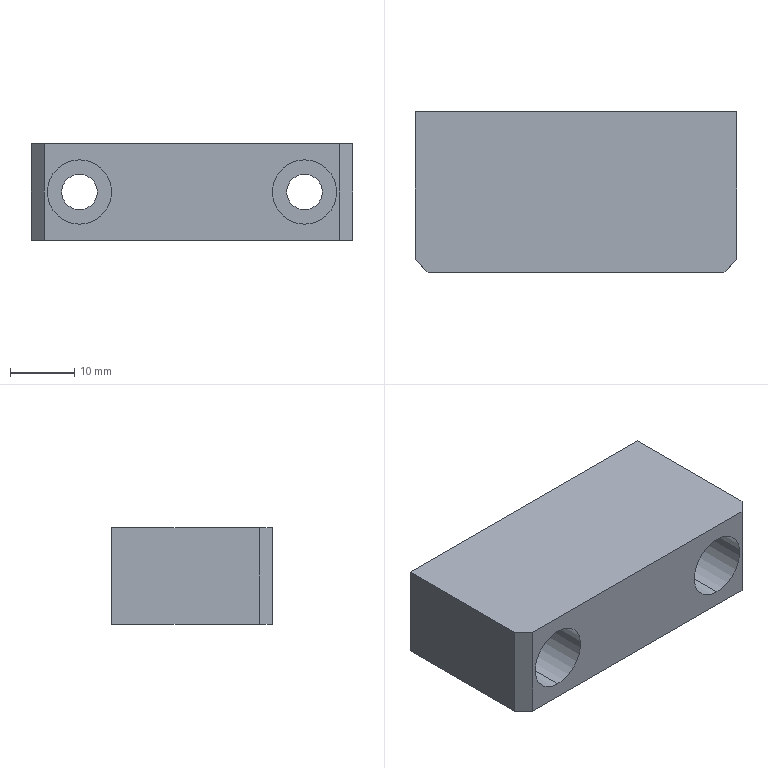Part | SolidWorks | features Chamfer 1, Extrusion 1, HoleWzd 1 | 1 solid | 18 faces | box 50 x 25 x 15 mm | volume 15782 mm3 | plane 10 | cylinder 8 | commonest cylinder face diameters 5.5 x4 10 x4
STEP:
#1=CARTESIAN_POINT('',(17.5,3.2,12.5));
#2=VERTEX_POINT('',#1);
#3=CARTESIAN_POINT('',(17.5,3.2,2.5));
#4=VERTEX_POINT('',#3);
#5=CARTESIAN_POINT('',(17.5,3.2,7.5));
#6=DIRECTION('',(0.,-1.,0.));
#7=DIRECTION('',(0.,0.,-1.));
#8=AXIS2_PLACEMENT_3D('',#5,#6,#7);
#9=CIRCLE('',#8,5.);
#10=EDGE_CURVE('',#2,#4,#9,.T.);
#11=ORIENTED_EDGE('',*,*,#10,.F.);
#12=CARTESIAN_POINT('',(17.5,-12.5,12.5));
#13=VERTEX_POINT('',#12);
#14=CARTESIAN_POINT('',(17.5,-12.5,12.5));
#15=DIRECTION('',(0.,-1.,0.));
#16=VECTOR('',#15,1000.);
#17=LINE('',#14,#16);
#18=EDGE_CURVE('',#2,#13,#17,.T.);
#19=ORIENTED_EDGE('',*,*,#18,.T.);
#20=CARTESIAN_POINT('',(17.5,-12.5,2.5));
#21=VERTEX_POINT('',#20);
#22=CARTESIAN_POINT('',(17.5,-12.5,7.5));
#23=DIRECTION('',(0.,-1.,0.));
#24=DIRECTION('',(0.,0.,-1.));
#25=AXIS2_PLACEMENT_3D('',#22,#23,#24);
#26=CIRCLE('',#25,5.);
#27=EDGE_CURVE('',#13,#21,#26,.T.);
#28=ORIENTED_EDGE('',*,*,#27,.T.);
#29=CARTESIAN_POINT('',(17.5,-12.5,2.5));
#30=DIRECTION('',(0.,-1.,0.));
#31=VECTOR('',#30,1000.);
#32=LINE('',#29,#31);
#33=EDGE_CURVE('',#4,#21,#32,.T.);
#34=ORIENTED_EDGE('',*,*,#33,.F.);
#35=EDGE_LOOP('',(#11,#19,#28,#34));
#36=FACE_OUTER_BOUND('',#35,.T.);
#37=CARTESIAN_POINT('',(17.5,-12.5,7.5));
#38=DIRECTION('',(0.,-1.,0.));
#39=DIRECTION('',(0.,0.,-1.));
#40=AXIS2_PLACEMENT_3D('',#37,#38,#39);
#41=CYLINDRICAL_SURFACE('',#40,5.);
#42=ADVANCED_FACE('',(#36),#41,.F.);
#43=CARTESIAN_POINT('',(17.5,12.5,10.25));
#44=VERTEX_POINT('',#43);
#45=CARTESIAN_POINT('',(17.5,12.5,4.75));
#46=VERTEX_POINT('',#45);
#47=CARTESIAN_POINT('',(17.5,12.5,7.5));
#48=DIRECTION('',(0.,-1.,0.));
#49=DIRECTION('',(0.,0.,-1.));
#50=AXIS2_PLACEMENT_3D('',#47,#48,#49);
#51=CIRCLE('',#50,2.75);
#52=EDGE_CURVE('',#44,#46,#51,.T.);
#53=ORIENTED_EDGE('',*,*,#52,.F.);
#54=CARTESIAN_POINT('',(17.5,3.2,10.25));
#55=VERTEX_POINT('',#54);
#56=CARTESIAN_POINT('',(17.5,-12.5,10.25));
#57=DIRECTION('',(0.,-1.,0.));
#58=VECTOR('',#57,1000.);
#59=LINE('',#56,#58);
#60=EDGE_CURVE('',#44,#55,#59,.T.);
#61=ORIENTED_EDGE('',*,*,#60,.T.);
#62=CARTESIAN_POINT('',(17.5,3.2,4.75));
#63=VERTEX_POINT('',#62);
#64=CARTESIAN_POINT('',(17.5,3.2,7.5));
#65=DIRECTION('',(0.,-1.,0.));
#66=DIRECTION('',(0.,0.,-1.));
#67=AXIS2_PLACEMENT_3D('',#64,#65,#66);
#68=CIRCLE('',#67,2.75);
#69=EDGE_CURVE('',#55,#63,#68,.T.);
#70=ORIENTED_EDGE('',*,*,#69,.T.);
#71=CARTESIAN_POINT('',(17.5,-12.5,4.75));
#72=DIRECTION('',(0.,-1.,0.));
#73=VECTOR('',#72,1000.);
#74=LINE('',#71,#73);
#75=EDGE_CURVE('',#46,#63,#74,.T.);
#76=ORIENTED_EDGE('',*,*,#75,.F.);
#77=EDGE_LOOP('',(#53,#61,#70,#76));
#78=FACE_OUTER_BOUND('',#77,.T.);
#79=CARTESIAN_POINT('',(17.5,-12.5,7.5));
#80=DIRECTION('',(0.,-1.,0.));
#81=DIRECTION('',(0.,0.,-1.));
#82=AXIS2_PLACEMENT_3D('',#79,#80,#81);
#83=CYLINDRICAL_SURFACE('',#82,2.75);
#84=ADVANCED_FACE('',(#78),#83,.F.);
#85=CARTESIAN_POINT('',(-17.5,3.2,12.5));
#86=VERTEX_POINT('',#85);
#87=CARTESIAN_POINT('',(-17.5,3.2,2.5));
#88=VERTEX_POINT('',#87);
#89=CARTESIAN_POINT('',(-17.5,3.2,7.5));
#90=DIRECTION('',(0.,-1.,0.));
#91=DIRECTION('',(0.,0.,-1.));
#92=AXIS2_PLACEMENT_3D('',#89,#90,#91);
#93=CIRCLE('',#92,5.);
#94=EDGE_CURVE('',#86,#88,#93,.T.);
#95=ORIENTED_EDGE('',*,*,#94,.F.);
#96=CARTESIAN_POINT('',(-17.5,-12.5,12.5));
#97=VERTEX_POINT('',#96);
#98=CARTESIAN_POINT('',(-17.5,-12.5,12.5));
#99=DIRECTION('',(0.,-1.,0.));
#100=VECTOR('',#99,1000.);
#101=LINE('',#98,#100);
#102=EDGE_CURVE('',#86,#97,#101,.T.);
#103=ORIENTED_EDGE('',*,*,#102,.T.);
#104=CARTESIAN_POINT('',(-17.5,-12.5,2.5));
#105=VERTEX_POINT('',#104);
#106=CARTESIAN_POINT('',(-17.5,-12.5,7.5));
#107=DIRECTION('',(0.,-1.,0.));
#108=DIRECTION('',(0.,0.,-1.));
#109=AXIS2_PLACEMENT_3D('',#106,#107,#108);
#110=CIRCLE('',#109,5.);
#111=EDGE_CURVE('',#97,#105,#110,.T.);
#112=ORIENTED_EDGE('',*,*,#111,.T.);
#113=CARTESIAN_POINT('',(-17.5,-12.5,2.5));
#114=DIRECTION('',(0.,-1.,0.));
#115=VECTOR('',#114,1000.);
#116=LINE('',#113,#115);
#117=EDGE_CURVE('',#88,#105,#116,.T.);
#118=ORIENTED_EDGE('',*,*,#117,.F.);
#119=EDGE_LOOP('',(#95,#103,#112,#118));
#120=FACE_OUTER_BOUND('',#119,.T.);
#121=CARTESIAN_POINT('',(-17.5,-12.5,7.5));
#122=DIRECTION('',(0.,-1.,0.));
#123=DIRECTION('',(0.,0.,-1.));
#124=AXIS2_PLACEMENT_3D('',#121,#122,#123);
#125=CYLINDRICAL_SURFACE('',#124,5.);
#126=ADVANCED_FACE('',(#120),#125,.F.);
#127=CARTESIAN_POINT('',(-17.5,12.5,10.25));
#128=VERTEX_POINT('',#127);
#129=CARTESIAN_POINT('',(-17.5,12.5,4.75));
#130=VERTEX_POINT('',#129);
#131=CARTESIAN_POINT('',(-17.5,12.5,7.5));
#132=DIRECTION('',(0.,-1.,0.));
#133=DIRECTION('',(0.,0.,-1.));
#134=AXIS2_PLACEMENT_3D('',#131,#132,#133);
#135=CIRCLE('',#134,2.75);
#136=EDGE_CURVE('',#128,#130,#135,.T.);
#137=ORIENTED_EDGE('',*,*,#136,.F.);
#138=CARTESIAN_POINT('',(-17.5,3.2,10.25));
#139=VERTEX_POINT('',#138);
#140=CARTESIAN_POINT('',(-17.5,-12.5,10.25));
#141=DIRECTION('',(0.,-1.,0.));
#142=VECTOR('',#141,1000.);
#143=LINE('',#140,#142);
#144=EDGE_CURVE('',#128,#139,#143,.T.);
#145=ORIENTED_EDGE('',*,*,#144,.T.);
#146=CARTESIAN_POINT('',(-17.5,3.2,4.75));
#147=VERTEX_POINT('',#146);
#148=CARTESIAN_POINT('',(-17.5,3.2,7.5));
#149=DIRECTION('',(0.,-1.,0.));
#150=DIRECTION('',(0.,0.,-1.));
#151=AXIS2_PLACEMENT_3D('',#148,#149,#150);
#152=CIRCLE('',#151,2.75);
#153=EDGE_CURVE('',#139,#147,#152,.T.);
#154=ORIENTED_EDGE('',*,*,#153,.T.);
#155=CARTESIAN_POINT('',(-17.5,-12.5,4.75));
#156=DIRECTION('',(0.,-1.,0.));
#157=VECTOR('',#156,1000.);
#158=LINE('',#155,#157);
#159=EDGE_CURVE('',#130,#147,#158,.T.);
#160=ORIENTED_EDGE('',*,*,#159,.F.);
#161=EDGE_LOOP('',(#137,#145,#154,#160));
#162=FACE_OUTER_BOUND('',#161,.T.);
#163=CARTESIAN_POINT('',(-17.5,-12.5,7.5));
#164=DIRECTION('',(0.,-1.,0.));
#165=DIRECTION('',(0.,0.,-1.));
#166=AXIS2_PLACEMENT_3D('',#163,#164,#165);
#167=CYLINDRICAL_SURFACE('',#166,2.75);
#168=ADVANCED_FACE('',(#162),#167,.F.);
#169=CARTESIAN_POINT('',(25.,-10.5,15.));
#170=VERTEX_POINT('',#169);
#171=CARTESIAN_POINT('',(25.,12.5,15.));
#172=VERTEX_POINT('',#171);
#173=CARTESIAN_POINT('',(25.,-12.5,15.));
#174=DIRECTION('',(0.,1.,0.));
#175=VECTOR('',#174,1000.);
#176=LINE('',#173,#175);
#177=EDGE_CURVE('',#170,#172,#176,.T.);
#178=ORIENTED_EDGE('',*,*,#177,.F.);
#179=CARTESIAN_POINT('',(25.,-10.5,0.));
#180=VERTEX_POINT('',#179);
#181=CARTESIAN_POINT('',(25.,-10.5,15.));
#182=DIRECTION('',(0.,0.,-1.));
#183=VECTOR('',#182,1000.);
#184=LINE('',#181,#183);
#185=EDGE_CURVE('',#170,#180,#184,.T.);
#186=ORIENTED_EDGE('',*,*,#185,.T.);
#187=CARTESIAN_POINT('',(25.,12.5,0.));
#188=VERTEX_POINT('',#187);
#189=CARTESIAN_POINT('',(25.,-12.5,0.));
#190=DIRECTION('',(0.,1.,0.));
#191=VECTOR('',#190,1000.);
#192=LINE('',#189,#191);
#193=EDGE_CURVE('',#180,#188,#192,.T.);
#194=ORIENTED_EDGE('',*,*,#193,.T.);
#195=CARTESIAN_POINT('',(25.,12.5,15.));
#196=DIRECTION('',(0.,0.,-1.));
#197=VECTOR('',#196,1000.);
#198=LINE('',#195,#197);
#199=EDGE_CURVE('',#172,#188,#198,.T.);
#200=ORIENTED_EDGE('',*,*,#199,.F.);
#201=EDGE_LOOP('',(#178,#186,#194,#200));
#202=FACE_OUTER_BOUND('',#201,.T.);
#203=CARTESIAN_POINT('',(25.,-12.5,15.));
#204=DIRECTION('',(-1.,0.,0.));
#205=DIRECTION('',(0.,0.,1.));
#206=AXIS2_PLACEMENT_3D('',#203,#204,#205);
#207=PLANE('',#206);
#208=ADVANCED_FACE('',(#202),#207,.F.);
#209=CARTESIAN_POINT('',(17.5,12.5,7.5));
#210=DIRECTION('',(0.,-1.,0.));
#211=DIRECTION('',(0.,0.,-1.));
#212=AXIS2_PLACEMENT_3D('',#209,#210,#211);
#213=CIRCLE('',#212,2.75);
#214=EDGE_CURVE('',#46,#44,#213,.T.);
#215=ORIENTED_EDGE('',*,*,#214,.T.);
#216=ORIENTED_EDGE('',*,*,#52,.T.);
#217=EDGE_LOOP('',(#215,#216));
#218=FACE_BOUND('',#217,.T.);
#219=CARTESIAN_POINT('',(-17.5,12.5,7.5));
#220=DIRECTION('',(0.,-1.,0.));
#221=DIRECTION('',(0.,0.,-1.));
#222=AXIS2_PLACEMENT_3D('',#219,#220,#221);
#223=CIRCLE('',#222,2.75);
#224=EDGE_CURVE('',#130,#128,#223,.T.);
#225=ORIENTED_EDGE('',*,*,#224,.T.);
#226=ORIENTED_EDGE('',*,*,#136,.T.);
#227=EDGE_LOOP('',(#225,#226));
#228=FACE_BOUND('',#227,.T.);
#229=CARTESIAN_POINT('',(-25.,12.5,0.));
#230=VERTEX_POINT('',#229);
#231=CARTESIAN_POINT('',(-25.,12.5,0.));
#232=DIRECTION('',(-1.,0.,0.));
#233=VECTOR('',#232,1000.);
#234=LINE('',#231,#233);
#235=EDGE_CURVE('',#188,#230,#234,.T.);
#236=ORIENTED_EDGE('',*,*,#235,.T.);
#237=CARTESIAN_POINT('',(-25.,12.5,15.));
#238=VERTEX_POINT('',#237);
#239=CARTESIAN_POINT('',(-25.,12.5,15.));
#240=DIRECTION('',(0.,0.,-1.));
#241=VECTOR('',#240,1000.);
#242=LINE('',#239,#241);
#243=EDGE_CURVE('',#238,#230,#242,.T.);
#244=ORIENTED_EDGE('',*,*,#243,.F.);
#245=CARTESIAN_POINT('',(-25.,12.5,15.));
#246=DIRECTION('',(-1.,0.,0.));
#247=VECTOR('',#246,1000.);
#248=LINE('',#245,#247);
#249=EDGE_CURVE('',#172,#238,#248,.T.);
#250=ORIENTED_EDGE('',*,*,#249,.F.);
#251=ORIENTED_EDGE('',*,*,#199,.T.);
#252=EDGE_LOOP('',(#236,#244,#250,#251));
#253=FACE_OUTER_BOUND('',#252,.T.);
#254=CARTESIAN_POINT('',(-25.,12.5,15.));
#255=DIRECTION('',(0.,-1.,0.));
#256=DIRECTION('',(0.,0.,-1.));
#257=AXIS2_PLACEMENT_3D('',#254,#255,#256);
#258=PLANE('',#257);
#259=ADVANCED_FACE('',(#218,#228,#253),#258,.F.);
#260=CARTESIAN_POINT('',(-25.,-10.5,0.));
#261=VERTEX_POINT('',#260);
#262=CARTESIAN_POINT('',(-25.,-12.5,0.));
#263=DIRECTION('',(0.,-1.,0.));
#264=VECTOR('',#263,1000.);
#265=LINE('',#262,#264);
#266=EDGE_CURVE('',#230,#261,#265,.T.);
#267=ORIENTED_EDGE('',*,*,#266,.T.);
#268=CARTESIAN_POINT('',(-25.,-10.5,15.));
#269=VERTEX_POINT('',#268);
#270=CARTESIAN_POINT('',(-25.,-10.5,15.));
#271=DIRECTION('',(0.,0.,1.));
#272=VECTOR('',#271,1000.);
#273=LINE('',#270,#272);
#274=EDGE_CURVE('',#261,#269,#273,.T.);
#275=ORIENTED_EDGE('',*,*,#274,.T.);
#276=CARTESIAN_POINT('',(-25.,-12.5,15.));
#277=DIRECTION('',(0.,-1.,0.));
#278=VECTOR('',#277,1000.);
#279=LINE('',#276,#278);
#280=EDGE_CURVE('',#238,#269,#279,.T.);
#281=ORIENTED_EDGE('',*,*,#280,.F.);
#282=ORIENTED_EDGE('',*,*,#243,.T.);
#283=EDGE_LOOP('',(#267,#275,#281,#282));
#284=FACE_OUTER_BOUND('',#283,.T.);
#285=CARTESIAN_POINT('',(-25.,-12.5,15.));
#286=DIRECTION('',(1.,0.,0.));
#287=DIRECTION('',(0.,0.,-1.));
#288=AXIS2_PLACEMENT_3D('',#285,#286,#287);
#289=PLANE('',#288);
#290=ADVANCED_FACE('',(#284),#289,.F.);
#291=CARTESIAN_POINT('',(17.5,-12.5,7.5));
#292=DIRECTION('',(0.,-1.,0.));
#293=DIRECTION('',(0.,0.,-1.));
#294=AXIS2_PLACEMENT_3D('',#291,#292,#293);
#295=CIRCLE('',#294,5.);
#296=EDGE_CURVE('',#21,#13,#295,.T.);
#297=ORIENTED_EDGE('',*,*,#296,.F.);
#298=ORIENTED_EDGE('',*,*,#27,.F.);
#299=EDGE_LOOP('',(#297,#298));
#300=FACE_BOUND('',#299,.T.);
#301=CARTESIAN_POINT('',(-17.5,-12.5,7.5));
#302=DIRECTION('',(0.,-1.,0.));
#303=DIRECTION('',(0.,0.,-1.));
#304=AXIS2_PLACEMENT_3D('',#301,#302,#303);
#305=CIRCLE('',#304,5.);
#306=EDGE_CURVE('',#105,#97,#305,.T.);
#307=ORIENTED_EDGE('',*,*,#306,.F.);
#308=ORIENTED_EDGE('',*,*,#111,.F.);
#309=EDGE_LOOP('',(#307,#308));
#310=FACE_BOUND('',#309,.T.);
#311=CARTESIAN_POINT('',(-23.,-12.5,0.));
#312=VERTEX_POINT('',#311);
#313=CARTESIAN_POINT('',(23.,-12.5,0.));
#314=VERTEX_POINT('',#313);
#315=CARTESIAN_POINT('',(-25.,-12.5,0.));
#316=DIRECTION('',(1.,0.,0.));
#317=VECTOR('',#316,1000.);
#318=LINE('',#315,#317);
#319=EDGE_CURVE('',#312,#314,#318,.T.);
#320=ORIENTED_EDGE('',*,*,#319,.T.);
#321=CARTESIAN_POINT('',(23.,-12.5,15.));
#322=VERTEX_POINT('',#321);
#323=CARTESIAN_POINT('',(23.,-12.5,15.));
#324=DIRECTION('',(0.,0.,1.));
#325=VECTOR('',#324,1000.);
#326=LINE('',#323,#325);
#327=EDGE_CURVE('',#314,#322,#326,.T.);
#328=ORIENTED_EDGE('',*,*,#327,.T.);
#329=CARTESIAN_POINT('',(-23.,-12.5,15.));
#330=VERTEX_POINT('',#329);
#331=CARTESIAN_POINT('',(-25.,-12.5,15.));
#332=DIRECTION('',(1.,0.,0.));
#333=VECTOR('',#332,1000.);
#334=LINE('',#331,#333);
#335=EDGE_CURVE('',#330,#322,#334,.T.);
#336=ORIENTED_EDGE('',*,*,#335,.F.);
#337=CARTESIAN_POINT('',(-23.,-12.5,15.));
#338=DIRECTION('',(0.,0.,-1.));
#339=VECTOR('',#338,1000.);
#340=LINE('',#337,#339);
#341=EDGE_CURVE('',#330,#312,#340,.T.);
#342=ORIENTED_EDGE('',*,*,#341,.T.);
#343=EDGE_LOOP('',(#320,#328,#336,#342));
#344=FACE_OUTER_BOUND('',#343,.T.);
#345=CARTESIAN_POINT('',(-25.,-12.5,15.));
#346=DIRECTION('',(0.,1.,0.));
#347=DIRECTION('',(0.,0.,1.));
#348=AXIS2_PLACEMENT_3D('',#345,#346,#347);
#349=PLANE('',#348);
#350=ADVANCED_FACE('',(#300,#310,#344),#349,.F.);
#351=ORIENTED_EDGE('',*,*,#335,.T.);
#352=CARTESIAN_POINT('',(25.,-10.5,15.));
#353=DIRECTION('',(0.7071,0.7071,0.));
#354=VECTOR('',#353,1000.);
#355=LINE('',#352,#354);
#356=EDGE_CURVE('',#322,#170,#355,.T.);
#357=ORIENTED_EDGE('',*,*,#356,.T.);
#358=ORIENTED_EDGE('',*,*,#177,.T.);
#359=ORIENTED_EDGE('',*,*,#249,.T.);
#360=ORIENTED_EDGE('',*,*,#280,.T.);
#361=CARTESIAN_POINT('',(-23.,-12.5,15.));
#362=DIRECTION('',(0.7071,-0.7071,0.));
#363=VECTOR('',#362,1000.);
#364=LINE('',#361,#363);
#365=EDGE_CURVE('',#269,#330,#364,.T.);
#366=ORIENTED_EDGE('',*,*,#365,.T.);
#367=EDGE_LOOP('',(#351,#357,#358,#359,#360,#366));
#368=FACE_OUTER_BOUND('',#367,.T.);
#369=CARTESIAN_POINT('',(0.,0.,15.));
#370=DIRECTION('',(0.,0.,-1.));
#371=DIRECTION('',(-1.,0.,0.));
#372=AXIS2_PLACEMENT_3D('',#369,#370,#371);
#373=PLANE('',#372);
#374=ADVANCED_FACE('',(#368),#373,.F.);
#375=ORIENTED_EDGE('',*,*,#193,.F.);
#376=CARTESIAN_POINT('',(17.75,-17.75,0.));
#377=DIRECTION('',(-0.7071,-0.7071,0.));
#378=VECTOR('',#377,1000.);
#379=LINE('',#376,#378);
#380=EDGE_CURVE('',#180,#314,#379,.T.);
#381=ORIENTED_EDGE('',*,*,#380,.T.);
#382=ORIENTED_EDGE('',*,*,#319,.F.);
#383=CARTESIAN_POINT('',(-17.75,-17.75,0.));
#384=DIRECTION('',(-0.7071,0.7071,0.));
#385=VECTOR('',#384,1000.);
#386=LINE('',#383,#385);
#387=EDGE_CURVE('',#312,#261,#386,.T.);
#388=ORIENTED_EDGE('',*,*,#387,.T.);
#389=ORIENTED_EDGE('',*,*,#266,.F.);
#390=ORIENTED_EDGE('',*,*,#235,.F.);
#391=EDGE_LOOP('',(#375,#381,#382,#388,#389,#390));
#392=FACE_OUTER_BOUND('',#391,.T.);
#393=CARTESIAN_POINT('',(0.,0.,0.));
#394=DIRECTION('',(0.,0.,-1.));
#395=DIRECTION('',(-1.,0.,0.));
#396=AXIS2_PLACEMENT_3D('',#393,#394,#395);
#397=PLANE('',#396);
#398=ADVANCED_FACE('',(#392),#397,.T.);
#399=ORIENTED_EDGE('',*,*,#356,.F.);
#400=ORIENTED_EDGE('',*,*,#327,.F.);
#401=ORIENTED_EDGE('',*,*,#380,.F.);
#402=ORIENTED_EDGE('',*,*,#185,.F.);
#403=EDGE_LOOP('',(#399,#400,#401,#402));
#404=FACE_OUTER_BOUND('',#403,.T.);
#405=CARTESIAN_POINT('',(25.,-10.5,15.));
#406=DIRECTION('',(-0.7071,0.7071,0.));
#407=DIRECTION('',(0.,0.,-1.));
#408=AXIS2_PLACEMENT_3D('',#405,#406,#407);
#409=PLANE('',#408);
#410=ADVANCED_FACE('',(#404),#409,.F.);
#411=ORIENTED_EDGE('',*,*,#365,.F.);
#412=ORIENTED_EDGE('',*,*,#274,.F.);
#413=ORIENTED_EDGE('',*,*,#387,.F.);
#414=ORIENTED_EDGE('',*,*,#341,.F.);
#415=EDGE_LOOP('',(#411,#412,#413,#414));
#416=FACE_OUTER_BOUND('',#415,.T.);
#417=CARTESIAN_POINT('',(-23.,-12.5,15.));
#418=DIRECTION('',(0.7071,0.7071,0.));
#419=DIRECTION('',(0.,0.,-1.));
#420=AXIS2_PLACEMENT_3D('',#417,#418,#419);
#421=PLANE('',#420);
#422=ADVANCED_FACE('',(#416),#421,.F.);
#423=ORIENTED_EDGE('',*,*,#144,.F.);
#424=ORIENTED_EDGE('',*,*,#224,.F.);
#425=ORIENTED_EDGE('',*,*,#159,.T.);
#426=CARTESIAN_POINT('',(-17.5,3.2,7.5));
#427=DIRECTION('',(0.,-1.,0.));
#428=DIRECTION('',(0.,0.,-1.));
#429=AXIS2_PLACEMENT_3D('',#426,#427,#428);
#430=CIRCLE('',#429,2.75);
#431=EDGE_CURVE('',#147,#139,#430,.T.);
#432=ORIENTED_EDGE('',*,*,#431,.T.);
#433=EDGE_LOOP('',(#423,#424,#425,#432));
#434=FACE_OUTER_BOUND('',#433,.T.);
#435=CARTESIAN_POINT('',(-17.5,-12.5,7.5));
#436=DIRECTION('',(0.,-1.,0.));
#437=DIRECTION('',(0.,0.,-1.));
#438=AXIS2_PLACEMENT_3D('',#435,#436,#437);
#439=CYLINDRICAL_SURFACE('',#438,2.75);
#440=ADVANCED_FACE('',(#434),#439,.F.);
#441=ORIENTED_EDGE('',*,*,#431,.F.);
#442=ORIENTED_EDGE('',*,*,#153,.F.);
#443=EDGE_LOOP('',(#441,#442));
#444=FACE_BOUND('',#443,.T.);
#445=CARTESIAN_POINT('',(-17.5,3.2,7.5));
#446=DIRECTION('',(0.,-1.,0.));
#447=DIRECTION('',(0.,0.,-1.));
#448=AXIS2_PLACEMENT_3D('',#445,#446,#447);
#449=CIRCLE('',#448,5.);
#450=EDGE_CURVE('',#88,#86,#449,.T.);
#451=ORIENTED_EDGE('',*,*,#450,.T.);
#452=ORIENTED_EDGE('',*,*,#94,.T.);
#453=EDGE_LOOP('',(#451,#452));
#454=FACE_OUTER_BOUND('',#453,.T.);
#455=CARTESIAN_POINT('',(-14.75,3.2,7.5));
#456=DIRECTION('',(0.,1.,0.));
#457=DIRECTION('',(0.,0.,1.));
#458=AXIS2_PLACEMENT_3D('',#455,#456,#457);
#459=PLANE('',#458);
#460=ADVANCED_FACE('',(#444,#454),#459,.F.);
#461=ORIENTED_EDGE('',*,*,#102,.F.);
#462=ORIENTED_EDGE('',*,*,#450,.F.);
#463=ORIENTED_EDGE('',*,*,#117,.T.);
#464=ORIENTED_EDGE('',*,*,#306,.T.);
#465=EDGE_LOOP('',(#461,#462,#463,#464));
#466=FACE_OUTER_BOUND('',#465,.T.);
#467=CARTESIAN_POINT('',(-17.5,-12.5,7.5));
#468=DIRECTION('',(0.,-1.,0.));
#469=DIRECTION('',(0.,0.,-1.));
#470=AXIS2_PLACEMENT_3D('',#467,#468,#469);
#471=CYLINDRICAL_SURFACE('',#470,5.);
#472=ADVANCED_FACE('',(#466),#471,.F.);
#473=ORIENTED_EDGE('',*,*,#60,.F.);
#474=ORIENTED_EDGE('',*,*,#214,.F.);
#475=ORIENTED_EDGE('',*,*,#75,.T.);
#476=CARTESIAN_POINT('',(17.5,3.2,7.5));
#477=DIRECTION('',(0.,-1.,0.));
#478=DIRECTION('',(0.,0.,-1.));
#479=AXIS2_PLACEMENT_3D('',#476,#477,#478);
#480=CIRCLE('',#479,2.75);
#481=EDGE_CURVE('',#63,#55,#480,.T.);
#482=ORIENTED_EDGE('',*,*,#481,.T.);
#483=EDGE_LOOP('',(#473,#474,#475,#482));
#484=FACE_OUTER_BOUND('',#483,.T.);
#485=CARTESIAN_POINT('',(17.5,-12.5,7.5));
#486=DIRECTION('',(0.,-1.,0.));
#487=DIRECTION('',(0.,0.,-1.));
#488=AXIS2_PLACEMENT_3D('',#485,#486,#487);
#489=CYLINDRICAL_SURFACE('',#488,2.75);
#490=ADVANCED_FACE('',(#484),#489,.F.);
#491=ORIENTED_EDGE('',*,*,#481,.F.);
#492=ORIENTED_EDGE('',*,*,#69,.F.);
#493=EDGE_LOOP('',(#491,#492));
#494=FACE_BOUND('',#493,.T.);
#495=CARTESIAN_POINT('',(17.5,3.2,7.5));
#496=DIRECTION('',(0.,-1.,0.));
#497=DIRECTION('',(0.,0.,-1.));
#498=AXIS2_PLACEMENT_3D('',#495,#496,#497);
#499=CIRCLE('',#498,5.);
#500=EDGE_CURVE('',#4,#2,#499,.T.);
#501=ORIENTED_EDGE('',*,*,#500,.T.);
#502=ORIENTED_EDGE('',*,*,#10,.T.);
#503=EDGE_LOOP('',(#501,#502));
#504=FACE_OUTER_BOUND('',#503,.T.);
#505=CARTESIAN_POINT('',(20.25,3.2,7.5));
#506=DIRECTION('',(0.,1.,0.));
#507=DIRECTION('',(0.,0.,1.));
#508=AXIS2_PLACEMENT_3D('',#505,#506,#507);
#509=PLANE('',#508);
#510=ADVANCED_FACE('',(#494,#504),#509,.F.);
#511=ORIENTED_EDGE('',*,*,#18,.F.);
#512=ORIENTED_EDGE('',*,*,#500,.F.);
#513=ORIENTED_EDGE('',*,*,#33,.T.);
#514=ORIENTED_EDGE('',*,*,#296,.T.);
#515=EDGE_LOOP('',(#511,#512,#513,#514));
#516=FACE_OUTER_BOUND('',#515,.T.);
#517=CARTESIAN_POINT('',(17.5,-12.5,7.5));
#518=DIRECTION('',(0.,-1.,0.));
#519=DIRECTION('',(0.,0.,-1.));
#520=AXIS2_PLACEMENT_3D('',#517,#518,#519);
#521=CYLINDRICAL_SURFACE('',#520,5.);
#522=ADVANCED_FACE('',(#516),#521,.F.);
#523=CLOSED_SHELL('',(#42,#84,#126,#168,#208,#259,#290,#350,#374,#398,#410,#422,#440,#460,#472,#490,#510,#522));
#524=MANIFOLD_SOLID_BREP('',#523);
#525=CARTESIAN_POINT('',(0.,0.,0.));
#526=DIRECTION('',(0.,0.,1.));
#527=DIRECTION('',(1.,0.,0.));
#528=AXIS2_PLACEMENT_3D('',#525,#526,#527);
#529=(LENGTH_UNIT()NAMED_UNIT(*)SI_UNIT(.MILLI.,.METRE.));
#530=UNCERTAINTY_MEASURE_WITH_UNIT(LENGTH_MEASURE(0.00001),#529,'','');
#531=(NAMED_UNIT(*)PLANE_ANGLE_UNIT()SI_UNIT($,.RADIAN.));
#532=(NAMED_UNIT(*)SI_UNIT($,.STERADIAN.)SOLID_ANGLE_UNIT());
#533=(GEOMETRIC_REPRESENTATION_CONTEXT(3)GLOBAL_UNCERTAINTY_ASSIGNED_CONTEXT((#530))GLOBAL_UNIT_ASSIGNED_CONTEXT((#529,#531,#532))REPRESENTATION_CONTEXT('',''));
#534=ADVANCED_BREP_SHAPE_REPRESENTATION('',(#524,#528),#533);